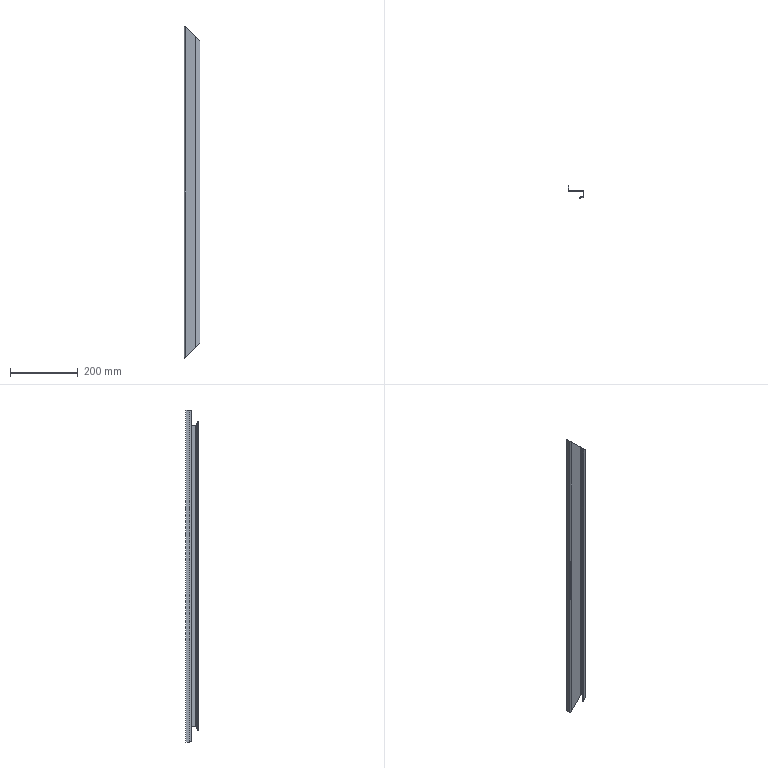Part | STEP file | 750038186 | 1 solid | 30 faces | box 47 x 35.779 x 981 mm | volume 158783 mm3 | plane 18 | cylinder 6 | spline 6 | commonest cylinder face diameters 4 x3 8 x3
STEP:
#1=CARTESIAN_POINT('',(43.,2.,-449.5));
#2=VERTEX_POINT('',#1);
#3=CARTESIAN_POINT('',(43.,2.,449.5));
#4=VERTEX_POINT('',#3);
#5=CARTESIAN_POINT('',(43.,2.,490.5));
#6=DIRECTION('',(0.,0.,1.));
#7=VECTOR('',#6,1000.);
#8=LINE('',#5,#7);
#9=EDGE_CURVE('',#2,#4,#8,.T.);
#10=ORIENTED_EDGE('',*,*,#9,.F.);
#11=CARTESIAN_POINT('',(4.,2.,-488.5));
#12=VERTEX_POINT('',#11);
#13=CARTESIAN_POINT('',(4.,2.,-488.5));
#14=DIRECTION('',(0.7071,0.,0.7071));
#15=VECTOR('',#14,1000.);
#16=LINE('',#13,#15);
#17=EDGE_CURVE('',#12,#2,#16,.T.);
#18=ORIENTED_EDGE('',*,*,#17,.F.);
#19=CARTESIAN_POINT('',(4.,2.,488.5));
#20=VERTEX_POINT('',#19);
#21=CARTESIAN_POINT('',(4.,2.,490.5));
#22=DIRECTION('',(0.,0.,-1.));
#23=VECTOR('',#22,1000.);
#24=LINE('',#21,#23);
#25=EDGE_CURVE('',#20,#12,#24,.T.);
#26=ORIENTED_EDGE('',*,*,#25,.F.);
#27=CARTESIAN_POINT('',(43.,2.,449.5));
#28=DIRECTION('',(-0.7071,0.,0.7071));
#29=VECTOR('',#28,1000.);
#30=LINE('',#27,#29);
#31=EDGE_CURVE('',#4,#20,#30,.T.);
#32=ORIENTED_EDGE('',*,*,#31,.F.);
#33=EDGE_LOOP('',(#10,#18,#26,#32));
#34=FACE_OUTER_BOUND('',#33,.T.);
#35=CARTESIAN_POINT('',(45.,2.,490.5));
#36=DIRECTION('',(0.,-1.,0.));
#37=DIRECTION('',(0.,0.,-1.));
#38=AXIS2_PLACEMENT_3D('',#35,#36,#37);
#39=PLANE('',#38);
#40=ADVANCED_FACE('',(#34),#39,.F.);
#41=CARTESIAN_POINT('',(43.,0.,449.5));
#42=VERTEX_POINT('',#41);
#43=CARTESIAN_POINT('',(43.,0.,449.5));
#44=DIRECTION('',(0.,1.,0.));
#45=VECTOR('',#44,1000.);
#46=LINE('',#43,#45);
#47=EDGE_CURVE('',#42,#4,#46,.T.);
#48=ORIENTED_EDGE('',*,*,#47,.T.);
#49=ORIENTED_EDGE('',*,*,#31,.T.);
#50=CARTESIAN_POINT('',(4.,0.,488.5));
#51=VERTEX_POINT('',#50);
#52=CARTESIAN_POINT('',(4.,0.,488.5));
#53=DIRECTION('',(0.,-1.,0.));
#54=VECTOR('',#53,1000.);
#55=LINE('',#52,#54);
#56=EDGE_CURVE('',#20,#51,#55,.T.);
#57=ORIENTED_EDGE('',*,*,#56,.T.);
#58=CARTESIAN_POINT('',(23.5,0.,469.));
#59=DIRECTION('',(0.7071,0.,-0.7071));
#60=VECTOR('',#59,1000.);
#61=LINE('',#58,#60);
#62=EDGE_CURVE('',#51,#42,#61,.T.);
#63=ORIENTED_EDGE('',*,*,#62,.T.);
#64=EDGE_LOOP('',(#48,#49,#57,#63));
#65=FACE_OUTER_BOUND('',#64,.T.);
#66=CARTESIAN_POINT('',(23.5,0.,469.));
#67=DIRECTION('',(0.7071,0.,0.7071));
#68=DIRECTION('',(0.7071,0.,-0.7071));
#69=AXIS2_PLACEMENT_3D('',#66,#67,#68);
#70=PLANE('',#69);
#71=ADVANCED_FACE('',(#65),#70,.T.);
#72=CARTESIAN_POINT('',(47.,-2.,-445.5));
#73=VERTEX_POINT('',#72);
#74=CARTESIAN_POINT('',(47.,-2.,-445.5));
#75=CARTESIAN_POINT('',(47.,0.,-445.5));
#76=CARTESIAN_POINT('',(45.667,2.,-446.833));
#77=CARTESIAN_POINT('',(43.,2.,-449.5));
#78=(BOUNDED_CURVE()B_SPLINE_CURVE(3,(#74,#75,#76,#77),.UNSPECIFIED.,.F.,.T.)B_SPLINE_CURVE_WITH_KNOTS((4,4),(0.,0.007635),.UNSPECIFIED.)CURVE()GEOMETRIC_REPRESENTATION_ITEM()RATIONAL_B_SPLINE_CURVE((1.,0.6667,0.5,0.5))REPRESENTATION_ITEM(''));
#79=EDGE_CURVE('',#73,#2,#78,.T.);
#80=ORIENTED_EDGE('',*,*,#79,.T.);
#81=ORIENTED_EDGE('',*,*,#9,.T.);
#82=CARTESIAN_POINT('',(47.,-2.,445.5));
#83=VERTEX_POINT('',#82);
#84=CARTESIAN_POINT('',(43.,2.,449.5));
#85=CARTESIAN_POINT('',(45.667,2.,446.833));
#86=CARTESIAN_POINT('',(47.,0.,445.5));
#87=CARTESIAN_POINT('',(47.,-2.,445.5));
#88=(BOUNDED_CURVE()B_SPLINE_CURVE(3,(#84,#85,#86,#87),.UNSPECIFIED.,.F.,.F.)B_SPLINE_CURVE_WITH_KNOTS((4,4),(0.,0.007567),.UNSPECIFIED.)CURVE()GEOMETRIC_REPRESENTATION_ITEM()RATIONAL_B_SPLINE_CURVE((0.5,0.5,0.6667,1.))REPRESENTATION_ITEM(''));
#89=EDGE_CURVE('',#4,#83,#88,.T.);
#90=ORIENTED_EDGE('',*,*,#89,.T.);
#91=CARTESIAN_POINT('',(47.,-2.,490.5));
#92=DIRECTION('',(0.,0.,-1.));
#93=VECTOR('',#92,1000.);
#94=LINE('',#91,#93);
#95=EDGE_CURVE('',#83,#73,#94,.T.);
#96=ORIENTED_EDGE('',*,*,#95,.T.);
#97=EDGE_LOOP('',(#80,#81,#90,#96));
#98=FACE_OUTER_BOUND('',#97,.T.);
#99=CARTESIAN_POINT('',(43.,-2.,490.5));
#100=DIRECTION('',(0.,0.,-1.));
#101=DIRECTION('',(-1.,0.,0.));
#102=AXIS2_PLACEMENT_3D('',#99,#100,#101);
#103=CYLINDRICAL_SURFACE('',#102,4.);
#104=ADVANCED_FACE('',(#98),#103,.T.);
#105=CARTESIAN_POINT('',(4.,0.,-488.5));
#106=VERTEX_POINT('',#105);
#107=CARTESIAN_POINT('',(4.,0.,-488.5));
#108=DIRECTION('',(0.,1.,0.));
#109=VECTOR('',#108,1000.);
#110=LINE('',#107,#109);
#111=EDGE_CURVE('',#106,#12,#110,.T.);
#112=ORIENTED_EDGE('',*,*,#111,.T.);
#113=ORIENTED_EDGE('',*,*,#17,.T.);
#114=CARTESIAN_POINT('',(43.,0.,-449.5));
#115=VERTEX_POINT('',#114);
#116=CARTESIAN_POINT('',(43.,0.,-449.5));
#117=DIRECTION('',(0.,-1.,0.));
#118=VECTOR('',#117,1000.);
#119=LINE('',#116,#118);
#120=EDGE_CURVE('',#2,#115,#119,.T.);
#121=ORIENTED_EDGE('',*,*,#120,.T.);
#122=CARTESIAN_POINT('',(514.,0.,21.5));
#123=DIRECTION('',(-0.7071,0.,-0.7071));
#124=VECTOR('',#123,1000.);
#125=LINE('',#122,#124);
#126=EDGE_CURVE('',#115,#106,#125,.T.);
#127=ORIENTED_EDGE('',*,*,#126,.T.);
#128=EDGE_LOOP('',(#112,#113,#121,#127));
#129=FACE_OUTER_BOUND('',#128,.T.);
#130=CARTESIAN_POINT('',(514.,0.,21.5));
#131=DIRECTION('',(0.7071,0.,-0.7071));
#132=DIRECTION('',(-0.7071,0.,-0.7071));
#133=AXIS2_PLACEMENT_3D('',#130,#131,#132);
#134=PLANE('',#133);
#135=ADVANCED_FACE('',(#129),#134,.T.);
#136=ORIENTED_EDGE('',*,*,#25,.T.);
#137=CARTESIAN_POINT('',(2.,4.,-490.5));
#138=VERTEX_POINT('',#137);
#139=CARTESIAN_POINT('',(2.,4.,-490.5));
#140=CARTESIAN_POINT('',(2.,3.,-490.5));
#141=CARTESIAN_POINT('',(2.667,2.,-489.833));
#142=CARTESIAN_POINT('',(4.,2.,-488.5));
#143=(BOUNDED_CURVE()B_SPLINE_CURVE(3,(#139,#140,#141,#142),.UNSPECIFIED.,.F.,.F.)B_SPLINE_CURVE_WITH_KNOTS((4,4),(0.,0.003806),.UNSPECIFIED.)CURVE()GEOMETRIC_REPRESENTATION_ITEM()RATIONAL_B_SPLINE_CURVE((1.,0.6667,0.5,0.5))REPRESENTATION_ITEM(''));
#144=EDGE_CURVE('',#138,#12,#143,.T.);
#145=ORIENTED_EDGE('',*,*,#144,.F.);
#146=CARTESIAN_POINT('',(2.,4.,490.5));
#147=VERTEX_POINT('',#146);
#148=CARTESIAN_POINT('',(2.,4.,490.5));
#149=DIRECTION('',(0.,0.,-1.));
#150=VECTOR('',#149,1000.);
#151=LINE('',#148,#150);
#152=EDGE_CURVE('',#147,#138,#151,.T.);
#153=ORIENTED_EDGE('',*,*,#152,.F.);
#154=CARTESIAN_POINT('',(4.,2.,488.5));
#155=CARTESIAN_POINT('',(2.667,2.,489.833));
#156=CARTESIAN_POINT('',(2.,3.,490.5));
#157=CARTESIAN_POINT('',(2.,4.,490.5));
#158=(BOUNDED_CURVE()B_SPLINE_CURVE(3,(#154,#155,#156,#157),.UNSPECIFIED.,.F.,.F.)B_SPLINE_CURVE_WITH_KNOTS((4,4),(0.,0.003785),.UNSPECIFIED.)CURVE()GEOMETRIC_REPRESENTATION_ITEM()RATIONAL_B_SPLINE_CURVE((0.5,0.5,0.6667,1.))REPRESENTATION_ITEM(''));
#159=EDGE_CURVE('',#20,#147,#158,.T.);
#160=ORIENTED_EDGE('',*,*,#159,.F.);
#161=EDGE_LOOP('',(#136,#145,#153,#160));
#162=FACE_OUTER_BOUND('',#161,.T.);
#163=CARTESIAN_POINT('',(4.,4.,490.5));
#164=DIRECTION('',(0.,0.,-1.));
#165=DIRECTION('',(-1.,0.,0.));
#166=AXIS2_PLACEMENT_3D('',#163,#164,#165);
#167=CYLINDRICAL_SURFACE('',#166,2.);
#168=ADVANCED_FACE('',(#162),#167,.F.);
#169=ORIENTED_EDGE('',*,*,#89,.F.);
#170=ORIENTED_EDGE('',*,*,#47,.F.);
#171=CARTESIAN_POINT('',(45.,-2.,445.5));
#172=VERTEX_POINT('',#171);
#173=CARTESIAN_POINT('',(45.,-2.,445.5));
#174=CARTESIAN_POINT('',(45.,-1.,445.5));
#175=CARTESIAN_POINT('',(44.333,0.,446.833));
#176=CARTESIAN_POINT('',(43.,0.,449.5));
#177=(BOUNDED_CURVE()B_SPLINE_CURVE(3,(#173,#174,#175,#176),.UNSPECIFIED.,.F.,.T.)B_SPLINE_CURVE_WITH_KNOTS((4,4),(0.,0.00529),.UNSPECIFIED.)CURVE()GEOMETRIC_REPRESENTATION_ITEM()RATIONAL_B_SPLINE_CURVE((1.,0.6667,0.5,0.5))REPRESENTATION_ITEM(''));
#178=EDGE_CURVE('',#172,#42,#177,.T.);
#179=ORIENTED_EDGE('',*,*,#178,.F.);
#180=CARTESIAN_POINT('',(46.,-2.,445.5));
#181=DIRECTION('',(-1.,0.,0.));
#182=VECTOR('',#181,1000.);
#183=LINE('',#180,#182);
#184=EDGE_CURVE('',#83,#172,#183,.T.);
#185=ORIENTED_EDGE('',*,*,#184,.F.);
#186=EDGE_LOOP('',(#169,#170,#179,#185));
#187=FACE_OUTER_BOUND('',#186,.T.);
#188=CARTESIAN_POINT('',(45.,-2.,445.5));
#189=CARTESIAN_POINT('',(45.667,-2.,445.5));
#190=CARTESIAN_POINT('',(46.333,-2.,445.5));
#191=CARTESIAN_POINT('',(47.,-2.,445.5));
#192=CARTESIAN_POINT('',(45.,2.,445.5));
#193=CARTESIAN_POINT('',(45.667,3.333,445.5));
#194=CARTESIAN_POINT('',(46.333,4.667,445.5));
#195=CARTESIAN_POINT('',(47.,6.,445.5));
#196=CARTESIAN_POINT('',(41.,2.,453.5));
#197=CARTESIAN_POINT('',(40.333,3.333,453.5));
#198=CARTESIAN_POINT('',(39.667,4.667,453.5));
#199=CARTESIAN_POINT('',(39.,6.,453.5));
#200=CARTESIAN_POINT('',(41.,-2.,453.5));
#201=CARTESIAN_POINT('',(40.333,-2.,453.5));
#202=CARTESIAN_POINT('',(39.667,-2.,453.5));
#203=CARTESIAN_POINT('',(39.,-2.,453.5));
#204=CARTESIAN_POINT('',(41.,-6.,453.5));
#205=CARTESIAN_POINT('',(40.333,-7.333,453.5));
#206=CARTESIAN_POINT('',(39.667,-8.667,453.5));
#207=CARTESIAN_POINT('',(39.,-10.,453.5));
#208=CARTESIAN_POINT('',(45.,-6.,445.5));
#209=CARTESIAN_POINT('',(45.667,-7.333,445.5));
#210=CARTESIAN_POINT('',(46.333,-8.667,445.5));
#211=CARTESIAN_POINT('',(47.,-10.,445.5));
#212=CARTESIAN_POINT('',(45.,-2.,445.5));
#213=CARTESIAN_POINT('',(45.667,-2.,445.5));
#214=CARTESIAN_POINT('',(46.333,-2.,445.5));
#215=CARTESIAN_POINT('',(47.,-2.,445.5));
#216=(BOUNDED_SURFACE()B_SPLINE_SURFACE(3,3,((#188,#189,#190,#191),(#192,#193,#194,#195),(#196,#197,#198,#199),(#200,#201,#202,#203),(#204,#205,#206,#207),(#208,#209,#210,#211),(#212,#213,#214,#215)),.UNSPECIFIED.,.T.,.F.,.F.)B_SPLINE_SURFACE_WITH_KNOTS((4,3,4),(4,4),(0.,0.5,1.),(0.,1.),.UNSPECIFIED.)GEOMETRIC_REPRESENTATION_ITEM()RATIONAL_B_SPLINE_SURFACE(((1.,1.,1.,1.),(0.3333,0.3333,0.3333,0.3333),(0.3333,0.3333,0.3333,0.3333),(1.,1.,1.,1.),(0.3333,0.3333,0.3333,0.3333),(0.3333,0.3333,0.3333,0.3333),(1.,1.,1.,1.)))REPRESENTATION_ITEM('')SURFACE());
#217=ADVANCED_FACE('',(#187),#216,.F.);
#218=CARTESIAN_POINT('',(4.,0.,490.5));
#219=DIRECTION('',(0.,0.,-1.));
#220=VECTOR('',#219,1000.);
#221=LINE('',#218,#220);
#222=EDGE_CURVE('',#51,#106,#221,.T.);
#223=ORIENTED_EDGE('',*,*,#222,.T.);
#224=ORIENTED_EDGE('',*,*,#126,.F.);
#225=CARTESIAN_POINT('',(43.,0.,490.5));
#226=DIRECTION('',(0.,0.,1.));
#227=VECTOR('',#226,1000.);
#228=LINE('',#225,#227);
#229=EDGE_CURVE('',#115,#42,#228,.T.);
#230=ORIENTED_EDGE('',*,*,#229,.T.);
#231=ORIENTED_EDGE('',*,*,#62,.F.);
#232=EDGE_LOOP('',(#223,#224,#230,#231));
#233=FACE_OUTER_BOUND('',#232,.T.);
#234=CARTESIAN_POINT('',(45.,0.,490.5));
#235=DIRECTION('',(0.,-1.,0.));
#236=DIRECTION('',(0.,0.,-1.));
#237=AXIS2_PLACEMENT_3D('',#234,#235,#236);
#238=PLANE('',#237);
#239=ADVANCED_FACE('',(#233),#238,.T.);
#240=ORIENTED_EDGE('',*,*,#56,.F.);
#241=ORIENTED_EDGE('',*,*,#159,.T.);
#242=CARTESIAN_POINT('',(0.,4.,490.5));
#243=VERTEX_POINT('',#242);
#244=CARTESIAN_POINT('',(1.,4.,490.5));
#245=DIRECTION('',(1.,0.,0.));
#246=VECTOR('',#245,1000.);
#247=LINE('',#244,#246);
#248=EDGE_CURVE('',#243,#147,#247,.T.);
#249=ORIENTED_EDGE('',*,*,#248,.F.);
#250=CARTESIAN_POINT('',(4.,0.,488.5));
#251=CARTESIAN_POINT('',(1.333,0.,489.833));
#252=CARTESIAN_POINT('',(0.,2.,490.5));
#253=CARTESIAN_POINT('',(0.,4.,490.5));
#254=(BOUNDED_CURVE()B_SPLINE_CURVE(3,(#250,#251,#252,#253),.UNSPECIFIED.,.F.,.T.)B_SPLINE_CURVE_WITH_KNOTS((4,4),(0.,0.006641),.UNSPECIFIED.)CURVE()GEOMETRIC_REPRESENTATION_ITEM()RATIONAL_B_SPLINE_CURVE((0.5,0.5,0.6667,1.))REPRESENTATION_ITEM(''));
#255=EDGE_CURVE('',#51,#243,#254,.T.);
#256=ORIENTED_EDGE('',*,*,#255,.F.);
#257=EDGE_LOOP('',(#240,#241,#249,#256));
#258=FACE_OUTER_BOUND('',#257,.T.);
#259=CARTESIAN_POINT('',(8.,4.,486.5));
#260=CARTESIAN_POINT('',(7.333,4.,486.5));
#261=CARTESIAN_POINT('',(6.667,4.,486.5));
#262=CARTESIAN_POINT('',(6.,4.,486.5));
#263=CARTESIAN_POINT('',(8.,-4.,486.5));
#264=CARTESIAN_POINT('',(7.333,-2.667,486.5));
#265=CARTESIAN_POINT('',(6.667,-1.333,486.5));
#266=CARTESIAN_POINT('',(6.,0.,486.5));
#267=CARTESIAN_POINT('',(0.,-4.,490.5));
#268=CARTESIAN_POINT('',(0.6667,-2.667,490.5));
#269=CARTESIAN_POINT('',(1.333,-1.333,490.5));
#270=CARTESIAN_POINT('',(2.,0.,490.5));
#271=CARTESIAN_POINT('',(0.,4.,490.5));
#272=CARTESIAN_POINT('',(0.6667,4.,490.5));
#273=CARTESIAN_POINT('',(1.333,4.,490.5));
#274=CARTESIAN_POINT('',(2.,4.,490.5));
#275=CARTESIAN_POINT('',(0.,12.,490.5));
#276=CARTESIAN_POINT('',(0.6667,10.667,490.5));
#277=CARTESIAN_POINT('',(1.333,9.333,490.5));
#278=CARTESIAN_POINT('',(2.,8.,490.5));
#279=CARTESIAN_POINT('',(8.,12.,486.5));
#280=CARTESIAN_POINT('',(7.333,10.667,486.5));
#281=CARTESIAN_POINT('',(6.667,9.333,486.5));
#282=CARTESIAN_POINT('',(6.,8.,486.5));
#283=CARTESIAN_POINT('',(8.,4.,486.5));
#284=CARTESIAN_POINT('',(7.333,4.,486.5));
#285=CARTESIAN_POINT('',(6.667,4.,486.5));
#286=CARTESIAN_POINT('',(6.,4.,486.5));
#287=(BOUNDED_SURFACE()B_SPLINE_SURFACE(3,3,((#259,#260,#261,#262),(#263,#264,#265,#266),(#267,#268,#269,#270),(#271,#272,#273,#274),(#275,#276,#277,#278),(#279,#280,#281,#282),(#283,#284,#285,#286)),.UNSPECIFIED.,.T.,.F.,.F.)B_SPLINE_SURFACE_WITH_KNOTS((4,3,4),(4,4),(0.,0.5,1.),(0.,1.),.UNSPECIFIED.)GEOMETRIC_REPRESENTATION_ITEM()RATIONAL_B_SPLINE_SURFACE(((1.,1.,1.,1.),(0.3333,0.3333,0.3333,0.3333),(0.3333,0.3333,0.3333,0.3333),(1.,1.,1.,1.),(0.3333,0.3333,0.3333,0.3333),(0.3333,0.3333,0.3333,0.3333),(1.,1.,1.,1.)))REPRESENTATION_ITEM('')SURFACE());
#288=ADVANCED_FACE('',(#258),#287,.F.);
#289=ORIENTED_EDGE('',*,*,#79,.F.);
#290=CARTESIAN_POINT('',(45.,-2.,-445.5));
#291=VERTEX_POINT('',#290);
#292=CARTESIAN_POINT('',(46.,-2.,-445.5));
#293=DIRECTION('',(1.,0.,0.));
#294=VECTOR('',#293,1000.);
#295=LINE('',#292,#294);
#296=EDGE_CURVE('',#291,#73,#295,.T.);
#297=ORIENTED_EDGE('',*,*,#296,.F.);
#298=CARTESIAN_POINT('',(43.,0.,-449.5));
#299=CARTESIAN_POINT('',(44.333,0.,-446.833));
#300=CARTESIAN_POINT('',(45.,-1.,-445.5));
#301=CARTESIAN_POINT('',(45.,-2.,-445.5));
#302=(BOUNDED_CURVE()B_SPLINE_CURVE(3,(#298,#299,#300,#301),.UNSPECIFIED.,.F.,.T.)B_SPLINE_CURVE_WITH_KNOTS((4,4),(0.,0.005228),.UNSPECIFIED.)CURVE()GEOMETRIC_REPRESENTATION_ITEM()RATIONAL_B_SPLINE_CURVE((0.5,0.5,0.6667,1.))REPRESENTATION_ITEM(''));
#303=EDGE_CURVE('',#115,#291,#302,.T.);
#304=ORIENTED_EDGE('',*,*,#303,.F.);
#305=ORIENTED_EDGE('',*,*,#120,.F.);
#306=EDGE_LOOP('',(#289,#297,#304,#305));
#307=FACE_OUTER_BOUND('',#306,.T.);
#308=CARTESIAN_POINT('',(41.,-2.,-453.5));
#309=CARTESIAN_POINT('',(40.333,-2.,-453.5));
#310=CARTESIAN_POINT('',(39.667,-2.,-453.5));
#311=CARTESIAN_POINT('',(39.,-2.,-453.5));
#312=CARTESIAN_POINT('',(41.,2.,-453.5));
#313=CARTESIAN_POINT('',(40.333,3.333,-453.5));
#314=CARTESIAN_POINT('',(39.667,4.667,-453.5));
#315=CARTESIAN_POINT('',(39.,6.,-453.5));
#316=CARTESIAN_POINT('',(45.,2.,-445.5));
#317=CARTESIAN_POINT('',(45.667,3.333,-445.5));
#318=CARTESIAN_POINT('',(46.333,4.667,-445.5));
#319=CARTESIAN_POINT('',(47.,6.,-445.5));
#320=CARTESIAN_POINT('',(45.,-2.,-445.5));
#321=CARTESIAN_POINT('',(45.667,-2.,-445.5));
#322=CARTESIAN_POINT('',(46.333,-2.,-445.5));
#323=CARTESIAN_POINT('',(47.,-2.,-445.5));
#324=CARTESIAN_POINT('',(45.,-6.,-445.5));
#325=CARTESIAN_POINT('',(45.667,-7.333,-445.5));
#326=CARTESIAN_POINT('',(46.333,-8.667,-445.5));
#327=CARTESIAN_POINT('',(47.,-10.,-445.5));
#328=CARTESIAN_POINT('',(41.,-6.,-453.5));
#329=CARTESIAN_POINT('',(40.333,-7.333,-453.5));
#330=CARTESIAN_POINT('',(39.667,-8.667,-453.5));
#331=CARTESIAN_POINT('',(39.,-10.,-453.5));
#332=CARTESIAN_POINT('',(41.,-2.,-453.5));
#333=CARTESIAN_POINT('',(40.333,-2.,-453.5));
#334=CARTESIAN_POINT('',(39.667,-2.,-453.5));
#335=CARTESIAN_POINT('',(39.,-2.,-453.5));
#336=(BOUNDED_SURFACE()B_SPLINE_SURFACE(3,3,((#308,#309,#310,#311),(#312,#313,#314,#315),(#316,#317,#318,#319),(#320,#321,#322,#323),(#324,#325,#326,#327),(#328,#329,#330,#331),(#332,#333,#334,#335)),.UNSPECIFIED.,.T.,.F.,.F.)B_SPLINE_SURFACE_WITH_KNOTS((4,3,4),(4,4),(0.,0.5,1.),(0.,1.),.UNSPECIFIED.)GEOMETRIC_REPRESENTATION_ITEM()RATIONAL_B_SPLINE_SURFACE(((1.,1.,1.,1.),(0.3333,0.3333,0.3333,0.3333),(0.3333,0.3333,0.3333,0.3333),(1.,1.,1.,1.),(0.3333,0.3333,0.3333,0.3333),(0.3333,0.3333,0.3333,0.3333),(1.,1.,1.,1.)))REPRESENTATION_ITEM('')SURFACE());
#337=ADVANCED_FACE('',(#307),#336,.F.);
#338=CARTESIAN_POINT('',(47.,-14.465,-445.5));
#339=VERTEX_POINT('',#338);
#340=CARTESIAN_POINT('',(47.,-14.465,445.5));
#341=VERTEX_POINT('',#340);
#342=CARTESIAN_POINT('',(47.,-14.465,490.5));
#343=DIRECTION('',(0.,0.,1.));
#344=VECTOR('',#343,1000.);
#345=LINE('',#342,#344);
#346=EDGE_CURVE('',#339,#341,#345,.T.);
#347=ORIENTED_EDGE('',*,*,#346,.F.);
#348=CARTESIAN_POINT('',(47.,-16.,-445.5));
#349=DIRECTION('',(0.,-1.,0.));
#350=VECTOR('',#349,1000.);
#351=LINE('',#348,#350);
#352=EDGE_CURVE('',#73,#339,#351,.T.);
#353=ORIENTED_EDGE('',*,*,#352,.F.);
#354=ORIENTED_EDGE('',*,*,#95,.F.);
#355=CARTESIAN_POINT('',(47.,-16.,445.5));
#356=DIRECTION('',(0.,1.,0.));
#357=VECTOR('',#356,1000.);
#358=LINE('',#355,#357);
#359=EDGE_CURVE('',#341,#83,#358,.T.);
#360=ORIENTED_EDGE('',*,*,#359,.F.);
#361=EDGE_LOOP('',(#347,#353,#354,#360));
#362=FACE_OUTER_BOUND('',#361,.T.);
#363=CARTESIAN_POINT('',(47.,-16.,490.5));
#364=DIRECTION('',(-1.,0.,0.));
#365=DIRECTION('',(0.,-1.,0.));
#366=AXIS2_PLACEMENT_3D('',#363,#364,#365);
#367=PLANE('',#366);
#368=ADVANCED_FACE('',(#362),#367,.F.);
#369=ORIENTED_EDGE('',*,*,#144,.T.);
#370=ORIENTED_EDGE('',*,*,#111,.F.);
#371=CARTESIAN_POINT('',(0.,4.,-490.5));
#372=VERTEX_POINT('',#371);
#373=CARTESIAN_POINT('',(0.,4.,-490.5));
#374=CARTESIAN_POINT('',(0.,2.,-490.5));
#375=CARTESIAN_POINT('',(1.333,0.,-489.833));
#376=CARTESIAN_POINT('',(4.,0.,-488.5));
#377=(BOUNDED_CURVE()B_SPLINE_CURVE(3,(#373,#374,#375,#376),.UNSPECIFIED.,.F.,.F.)B_SPLINE_CURVE_WITH_KNOTS((4,4),(0.,0.006627),.UNSPECIFIED.)CURVE()GEOMETRIC_REPRESENTATION_ITEM()RATIONAL_B_SPLINE_CURVE((1.,0.6667,0.5,0.5))REPRESENTATION_ITEM(''));
#378=EDGE_CURVE('',#372,#106,#377,.T.);
#379=ORIENTED_EDGE('',*,*,#378,.F.);
#380=CARTESIAN_POINT('',(1.,4.,-490.5));
#381=DIRECTION('',(-1.,0.,0.));
#382=VECTOR('',#381,1000.);
#383=LINE('',#380,#382);
#384=EDGE_CURVE('',#138,#372,#383,.T.);
#385=ORIENTED_EDGE('',*,*,#384,.F.);
#386=EDGE_LOOP('',(#369,#370,#379,#385));
#387=FACE_OUTER_BOUND('',#386,.T.);
#388=CARTESIAN_POINT('',(0.,4.,-490.5));
#389=CARTESIAN_POINT('',(0.6667,4.,-490.5));
#390=CARTESIAN_POINT('',(1.333,4.,-490.5));
#391=CARTESIAN_POINT('',(2.,4.,-490.5));
#392=CARTESIAN_POINT('',(0.,-4.,-490.5));
#393=CARTESIAN_POINT('',(0.6667,-2.667,-490.5));
#394=CARTESIAN_POINT('',(1.333,-1.333,-490.5));
#395=CARTESIAN_POINT('',(2.,0.,-490.5));
#396=CARTESIAN_POINT('',(8.,-4.,-486.5));
#397=CARTESIAN_POINT('',(7.333,-2.667,-486.5));
#398=CARTESIAN_POINT('',(6.667,-1.333,-486.5));
#399=CARTESIAN_POINT('',(6.,0.,-486.5));
#400=CARTESIAN_POINT('',(8.,4.,-486.5));
#401=CARTESIAN_POINT('',(7.333,4.,-486.5));
#402=CARTESIAN_POINT('',(6.667,4.,-486.5));
#403=CARTESIAN_POINT('',(6.,4.,-486.5));
#404=CARTESIAN_POINT('',(8.,12.,-486.5));
#405=CARTESIAN_POINT('',(7.333,10.667,-486.5));
#406=CARTESIAN_POINT('',(6.667,9.333,-486.5));
#407=CARTESIAN_POINT('',(6.,8.,-486.5));
#408=CARTESIAN_POINT('',(0.,12.,-490.5));
#409=CARTESIAN_POINT('',(0.6667,10.667,-490.5));
#410=CARTESIAN_POINT('',(1.333,9.333,-490.5));
#411=CARTESIAN_POINT('',(2.,8.,-490.5));
#412=CARTESIAN_POINT('',(0.,4.,-490.5));
#413=CARTESIAN_POINT('',(0.6667,4.,-490.5));
#414=CARTESIAN_POINT('',(1.333,4.,-490.5));
#415=CARTESIAN_POINT('',(2.,4.,-490.5));
#416=(BOUNDED_SURFACE()B_SPLINE_SURFACE(3,3,((#388,#389,#390,#391),(#392,#393,#394,#395),(#396,#397,#398,#399),(#400,#401,#402,#403),(#404,#405,#406,#407),(#408,#409,#410,#411),(#412,#413,#414,#415)),.UNSPECIFIED.,.T.,.F.,.T.)B_SPLINE_SURFACE_WITH_KNOTS((4,3,4),(4,4),(0.,0.5,1.),(0.,1.),.UNSPECIFIED.)GEOMETRIC_REPRESENTATION_ITEM()RATIONAL_B_SPLINE_SURFACE(((1.,1.,1.,1.),(0.3333,0.3333,0.3333,0.3333),(0.3333,0.3333,0.3333,0.3333),(1.,1.,1.,1.),(0.3333,0.3333,0.3333,0.3333),(0.3333,0.3333,0.3333,0.3333),(1.,1.,1.,1.)))REPRESENTATION_ITEM('')SURFACE());
#417=ADVANCED_FACE('',(#387),#416,.F.);
#418=CARTESIAN_POINT('',(2.,15.,490.5));
#419=VERTEX_POINT('',#418);
#420=CARTESIAN_POINT('',(2.,15.,-490.5));
#421=VERTEX_POINT('',#420);
#422=CARTESIAN_POINT('',(2.,15.,490.5));
#423=DIRECTION('',(0.,0.,-1.));
#424=VECTOR('',#423,1000.);
#425=LINE('',#422,#424);
#426=EDGE_CURVE('',#419,#421,#425,.T.);
#427=ORIENTED_EDGE('',*,*,#426,.F.);
#428=CARTESIAN_POINT('',(2.,0.,490.5));
#429=DIRECTION('',(0.,1.,0.));
#430=VECTOR('',#429,1000.);
#431=LINE('',#428,#430);
#432=EDGE_CURVE('',#147,#419,#431,.T.);
#433=ORIENTED_EDGE('',*,*,#432,.F.);
#434=ORIENTED_EDGE('',*,*,#152,.T.);
#435=CARTESIAN_POINT('',(2.,0.,-490.5));
#436=DIRECTION('',(0.,-1.,0.));
#437=VECTOR('',#436,1000.);
#438=LINE('',#435,#437);
#439=EDGE_CURVE('',#421,#138,#438,.T.);
#440=ORIENTED_EDGE('',*,*,#439,.F.);
#441=EDGE_LOOP('',(#427,#433,#434,#440));
#442=FACE_OUTER_BOUND('',#441,.T.);
#443=CARTESIAN_POINT('',(2.,0.,490.5));
#444=DIRECTION('',(-1.,0.,0.));
#445=DIRECTION('',(0.,-1.,0.));
#446=AXIS2_PLACEMENT_3D('',#443,#444,#445);
#447=PLANE('',#446);
#448=ADVANCED_FACE('',(#442),#447,.F.);
#449=ORIENTED_EDGE('',*,*,#184,.T.);
#450=CARTESIAN_POINT('',(45.,-14.465,445.5));
#451=VERTEX_POINT('',#450);
#452=CARTESIAN_POINT('',(45.,-16.,445.5));
#453=DIRECTION('',(0.,-1.,0.));
#454=VECTOR('',#453,1000.);
#455=LINE('',#452,#454);
#456=EDGE_CURVE('',#172,#451,#455,.T.);
#457=ORIENTED_EDGE('',*,*,#456,.T.);
#458=CARTESIAN_POINT('',(47.,-14.465,445.5));
#459=DIRECTION('',(1.,0.,0.));
#460=VECTOR('',#459,1000.);
#461=LINE('',#458,#460);
#462=EDGE_CURVE('',#451,#341,#461,.T.);
#463=ORIENTED_EDGE('',*,*,#462,.T.);
#464=ORIENTED_EDGE('',*,*,#359,.T.);
#465=EDGE_LOOP('',(#449,#457,#463,#464));
#466=FACE_OUTER_BOUND('',#465,.T.);
#467=CARTESIAN_POINT('',(47.,-16.,445.5));
#468=DIRECTION('',(0.,0.,1.));
#469=DIRECTION('',(0.,-1.,0.));
#470=AXIS2_PLACEMENT_3D('',#467,#468,#469);
#471=PLANE('',#470);
#472=ADVANCED_FACE('',(#466),#471,.T.);
#473=ORIENTED_EDGE('',*,*,#178,.T.);
#474=ORIENTED_EDGE('',*,*,#229,.F.);
#475=ORIENTED_EDGE('',*,*,#303,.T.);
#476=CARTESIAN_POINT('',(45.,-2.,490.5));
#477=DIRECTION('',(0.,0.,-1.));
#478=VECTOR('',#477,1000.);
#479=LINE('',#476,#478);
#480=EDGE_CURVE('',#172,#291,#479,.T.);
#481=ORIENTED_EDGE('',*,*,#480,.F.);
#482=EDGE_LOOP('',(#473,#474,#475,#481));
#483=FACE_OUTER_BOUND('',#482,.T.);
#484=CARTESIAN_POINT('',(43.,-2.,490.5));
#485=DIRECTION('',(0.,0.,-1.));
#486=DIRECTION('',(-1.,0.,0.));
#487=AXIS2_PLACEMENT_3D('',#484,#485,#486);
#488=CYLINDRICAL_SURFACE('',#487,2.);
#489=ADVANCED_FACE('',(#483),#488,.F.);
#490=CARTESIAN_POINT('',(0.,4.,490.5));
#491=DIRECTION('',(0.,0.,-1.));
#492=VECTOR('',#491,1000.);
#493=LINE('',#490,#492);
#494=EDGE_CURVE('',#243,#372,#493,.T.);
#495=ORIENTED_EDGE('',*,*,#494,.T.);
#496=ORIENTED_EDGE('',*,*,#378,.T.);
#497=ORIENTED_EDGE('',*,*,#222,.F.);
#498=ORIENTED_EDGE('',*,*,#255,.T.);
#499=EDGE_LOOP('',(#495,#496,#497,#498));
#500=FACE_OUTER_BOUND('',#499,.T.);
#501=CARTESIAN_POINT('',(4.,4.,490.5));
#502=DIRECTION('',(0.,0.,-1.));
#503=DIRECTION('',(-1.,0.,0.));
#504=AXIS2_PLACEMENT_3D('',#501,#502,#503);
#505=CYLINDRICAL_SURFACE('',#504,4.);
#506=ADVANCED_FACE('',(#500),#505,.T.);
#507=ORIENTED_EDGE('',*,*,#432,.T.);
#508=CARTESIAN_POINT('',(0.,15.,490.5));
#509=VERTEX_POINT('',#508);
#510=CARTESIAN_POINT('',(0.,15.,490.5));
#511=DIRECTION('',(-1.,0.,0.));
#512=VECTOR('',#511,1000.);
#513=LINE('',#510,#512);
#514=EDGE_CURVE('',#419,#509,#513,.T.);
#515=ORIENTED_EDGE('',*,*,#514,.T.);
#516=CARTESIAN_POINT('',(0.,0.,490.5));
#517=DIRECTION('',(0.,-1.,0.));
#518=VECTOR('',#517,1000.);
#519=LINE('',#516,#518);
#520=EDGE_CURVE('',#509,#243,#519,.T.);
#521=ORIENTED_EDGE('',*,*,#520,.T.);
#522=ORIENTED_EDGE('',*,*,#248,.T.);
#523=EDGE_LOOP('',(#507,#515,#521,#522));
#524=FACE_OUTER_BOUND('',#523,.T.);
#525=CARTESIAN_POINT('',(0.,0.,490.5));
#526=DIRECTION('',(0.,0.,1.));
#527=DIRECTION('',(1.,0.,0.));
#528=AXIS2_PLACEMENT_3D('',#525,#526,#527);
#529=PLANE('',#528);
#530=ADVANCED_FACE('',(#524),#529,.T.);
#531=CARTESIAN_POINT('',(45.,-14.465,-445.5));
#532=VERTEX_POINT('',#531);
#533=CARTESIAN_POINT('',(47.,-14.465,-445.5));
#534=DIRECTION('',(-1.,0.,0.));
#535=VECTOR('',#534,1000.);
#536=LINE('',#533,#535);
#537=EDGE_CURVE('',#339,#532,#536,.T.);
#538=ORIENTED_EDGE('',*,*,#537,.T.);
#539=CARTESIAN_POINT('',(45.,-16.,-445.5));
#540=DIRECTION('',(0.,1.,0.));
#541=VECTOR('',#540,1000.);
#542=LINE('',#539,#541);
#543=EDGE_CURVE('',#532,#291,#542,.T.);
#544=ORIENTED_EDGE('',*,*,#543,.T.);
#545=ORIENTED_EDGE('',*,*,#296,.T.);
#546=ORIENTED_EDGE('',*,*,#352,.T.);
#547=EDGE_LOOP('',(#538,#544,#545,#546));
#548=FACE_OUTER_BOUND('',#547,.T.);
#549=CARTESIAN_POINT('',(47.,-16.,-445.5));
#550=DIRECTION('',(0.,0.,-1.));
#551=DIRECTION('',(0.,1.,0.));
#552=AXIS2_PLACEMENT_3D('',#549,#550,#551);
#553=PLANE('',#552);
#554=ADVANCED_FACE('',(#548),#553,.T.);
#555=CARTESIAN_POINT('',(44.035,-18.329,-448.465));
#556=VERTEX_POINT('',#555);
#557=CARTESIAN_POINT('',(44.035,-18.329,-448.465));
#558=CARTESIAN_POINT('',(46.081,-17.781,-446.419));
#559=CARTESIAN_POINT('',(47.,-16.095,-445.5));
#560=CARTESIAN_POINT('',(47.,-14.465,-445.5));
#561=(BOUNDED_CURVE()B_SPLINE_CURVE(3,(#557,#558,#559,#560),.UNSPECIFIED.,.F.,.F.)B_SPLINE_CURVE_WITH_KNOTS((4,4),(0.,0.006101),.UNSPECIFIED.)CURVE()GEOMETRIC_REPRESENTATION_ITEM()RATIONAL_B_SPLINE_CURVE((0.5087,0.5468,0.7106,1.))REPRESENTATION_ITEM(''));
#562=EDGE_CURVE('',#556,#339,#561,.T.);
#563=ORIENTED_EDGE('',*,*,#562,.T.);
#564=ORIENTED_EDGE('',*,*,#346,.T.);
#565=CARTESIAN_POINT('',(44.035,-18.329,448.465));
#566=VERTEX_POINT('',#565);
#567=CARTESIAN_POINT('',(47.,-14.465,445.5));
#568=CARTESIAN_POINT('',(47.,-16.095,445.5));
#569=CARTESIAN_POINT('',(46.081,-17.781,446.419));
#570=CARTESIAN_POINT('',(44.035,-18.329,448.465));
#571=(BOUNDED_CURVE()B_SPLINE_CURVE(3,(#567,#568,#569,#570),.UNSPECIFIED.,.F.,.F.)B_SPLINE_CURVE_WITH_KNOTS((4,4),(0.,0.006218),.UNSPECIFIED.)CURVE()GEOMETRIC_REPRESENTATION_ITEM()RATIONAL_B_SPLINE_CURVE((1.,0.7106,0.5468,0.5087))REPRESENTATION_ITEM(''));
#572=EDGE_CURVE('',#341,#566,#571,.T.);
#573=ORIENTED_EDGE('',*,*,#572,.T.);
#574=CARTESIAN_POINT('',(44.035,-18.329,490.5));
#575=DIRECTION('',(0.,0.,-1.));
#576=VECTOR('',#575,1000.);
#577=LINE('',#574,#576);
#578=EDGE_CURVE('',#566,#556,#577,.T.);
#579=ORIENTED_EDGE('',*,*,#578,.T.);
#580=EDGE_LOOP('',(#563,#564,#573,#579));
#581=FACE_OUTER_BOUND('',#580,.T.);
#582=CARTESIAN_POINT('',(43.,-14.465,490.5));
#583=DIRECTION('',(0.,0.,-1.));
#584=DIRECTION('',(-1.,0.,0.));
#585=AXIS2_PLACEMENT_3D('',#582,#583,#584);
#586=CYLINDRICAL_SURFACE('',#585,4.);
#587=ADVANCED_FACE('',(#581),#586,.T.);
#588=CARTESIAN_POINT('',(0.,15.,-490.5));
#589=VERTEX_POINT('',#588);
#590=CARTESIAN_POINT('',(0.,-18.847,-490.5));
#591=DIRECTION('',(0.,-1.,0.));
#592=VECTOR('',#591,1000.);
#593=LINE('',#590,#592);
#594=EDGE_CURVE('',#589,#372,#593,.T.);
#595=ORIENTED_EDGE('',*,*,#594,.F.);
#596=CARTESIAN_POINT('',(34.375,15.,-490.5));
#597=DIRECTION('',(-1.,0.,0.));
#598=VECTOR('',#597,1000.);
#599=LINE('',#596,#598);
#600=EDGE_CURVE('',#421,#589,#599,.T.);
#601=ORIENTED_EDGE('',*,*,#600,.F.);
#602=ORIENTED_EDGE('',*,*,#439,.T.);
#603=ORIENTED_EDGE('',*,*,#384,.T.);
#604=EDGE_LOOP('',(#595,#601,#602,#603));
#605=FACE_OUTER_BOUND('',#604,.T.);
#606=CARTESIAN_POINT('',(34.375,-18.847,-490.5));
#607=DIRECTION('',(0.,0.,1.));
#608=DIRECTION('',(1.,0.,0.));
#609=AXIS2_PLACEMENT_3D('',#606,#607,#608);
#610=PLANE('',#609);
#611=ADVANCED_FACE('',(#605),#610,.F.);
#612=ORIENTED_EDGE('',*,*,#600,.T.);
#613=CARTESIAN_POINT('',(0.,15.,490.5));
#614=DIRECTION('',(0.,0.,1.));
#615=VECTOR('',#614,1000.);
#616=LINE('',#613,#615);
#617=EDGE_CURVE('',#589,#509,#616,.T.);
#618=ORIENTED_EDGE('',*,*,#617,.T.);
#619=ORIENTED_EDGE('',*,*,#514,.F.);
#620=ORIENTED_EDGE('',*,*,#426,.T.);
#621=EDGE_LOOP('',(#612,#618,#619,#620));
#622=FACE_OUTER_BOUND('',#621,.T.);
#623=CARTESIAN_POINT('',(0.,15.,490.5));
#624=DIRECTION('',(0.,1.,0.));
#625=DIRECTION('',(-1.,0.,0.));
#626=AXIS2_PLACEMENT_3D('',#623,#624,#625);
#627=PLANE('',#626);
#628=ADVANCED_FACE('',(#622),#627,.T.);
#629=ORIENTED_EDGE('',*,*,#480,.T.);
#630=ORIENTED_EDGE('',*,*,#543,.F.);
#631=CARTESIAN_POINT('',(45.,-14.465,490.5));
#632=DIRECTION('',(0.,0.,1.));
#633=VECTOR('',#632,1000.);
#634=LINE('',#631,#633);
#635=EDGE_CURVE('',#532,#451,#634,.T.);
#636=ORIENTED_EDGE('',*,*,#635,.T.);
#637=ORIENTED_EDGE('',*,*,#456,.F.);
#638=EDGE_LOOP('',(#629,#630,#636,#637));
#639=FACE_OUTER_BOUND('',#638,.T.);
#640=CARTESIAN_POINT('',(45.,-16.,490.5));
#641=DIRECTION('',(-1.,0.,0.));
#642=DIRECTION('',(0.,-1.,0.));
#643=AXIS2_PLACEMENT_3D('',#640,#641,#642);
#644=PLANE('',#643);
#645=ADVANCED_FACE('',(#639),#644,.T.);
#646=ORIENTED_EDGE('',*,*,#572,.F.);
#647=ORIENTED_EDGE('',*,*,#462,.F.);
#648=CARTESIAN_POINT('',(43.518,-16.397,448.465));
#649=VERTEX_POINT('',#648);
#650=CARTESIAN_POINT('',(43.518,-16.397,448.465));
#651=CARTESIAN_POINT('',(44.54,-16.123,446.419));
#652=CARTESIAN_POINT('',(45.,-15.28,445.5));
#653=CARTESIAN_POINT('',(45.,-14.465,445.5));
#654=(BOUNDED_CURVE()B_SPLINE_CURVE(3,(#650,#651,#652,#653),.UNSPECIFIED.,.F.,.F.)B_SPLINE_CURVE_WITH_KNOTS((4,4),(0.,0.004081),.UNSPECIFIED.)CURVE()GEOMETRIC_REPRESENTATION_ITEM()RATIONAL_B_SPLINE_CURVE((0.5087,0.5468,0.7106,1.))REPRESENTATION_ITEM(''));
#655=EDGE_CURVE('',#649,#451,#654,.T.);
#656=ORIENTED_EDGE('',*,*,#655,.F.);
#657=CARTESIAN_POINT('',(43.776,-17.363,448.465));
#658=DIRECTION('',(-0.2588,0.9659,0.));
#659=VECTOR('',#658,1000.);
#660=LINE('',#657,#659);
#661=EDGE_CURVE('',#566,#649,#660,.T.);
#662=ORIENTED_EDGE('',*,*,#661,.F.);
#663=EDGE_LOOP('',(#646,#647,#656,#662));
#664=FACE_OUTER_BOUND('',#663,.T.);
#665=CARTESIAN_POINT('',(45.,-14.465,445.5));
#666=CARTESIAN_POINT('',(45.667,-14.465,445.5));
#667=CARTESIAN_POINT('',(46.333,-14.465,445.5));
#668=CARTESIAN_POINT('',(47.,-14.465,445.5));
#669=CARTESIAN_POINT('',(45.,-10.465,445.5));
#670=CARTESIAN_POINT('',(45.667,-9.132,445.5));
#671=CARTESIAN_POINT('',(46.333,-7.799,445.5));
#672=CARTESIAN_POINT('',(47.,-6.465,445.5));
#673=CARTESIAN_POINT('',(41.,-10.465,453.5));
#674=CARTESIAN_POINT('',(40.333,-9.132,453.5));
#675=CARTESIAN_POINT('',(39.667,-7.799,453.5));
#676=CARTESIAN_POINT('',(39.,-6.465,453.5));
#677=CARTESIAN_POINT('',(41.,-14.465,453.5));
#678=CARTESIAN_POINT('',(40.333,-14.465,453.5));
#679=CARTESIAN_POINT('',(39.667,-14.465,453.5));
#680=CARTESIAN_POINT('',(39.,-14.465,453.5));
#681=CARTESIAN_POINT('',(41.,-18.465,453.5));
#682=CARTESIAN_POINT('',(40.333,-19.799,453.5));
#683=CARTESIAN_POINT('',(39.667,-21.132,453.5));
#684=CARTESIAN_POINT('',(39.,-22.465,453.5));
#685=CARTESIAN_POINT('',(45.,-18.465,445.5));
#686=CARTESIAN_POINT('',(45.667,-19.799,445.5));
#687=CARTESIAN_POINT('',(46.333,-21.132,445.5));
#688=CARTESIAN_POINT('',(47.,-22.465,445.5));
#689=CARTESIAN_POINT('',(45.,-14.465,445.5));
#690=CARTESIAN_POINT('',(45.667,-14.465,445.5));
#691=CARTESIAN_POINT('',(46.333,-14.465,445.5));
#692=CARTESIAN_POINT('',(47.,-14.465,445.5));
#693=(BOUNDED_SURFACE()B_SPLINE_SURFACE(3,3,((#665,#666,#667,#668),(#669,#670,#671,#672),(#673,#674,#675,#676),(#677,#678,#679,#680),(#681,#682,#683,#684),(#685,#686,#687,#688),(#689,#690,#691,#692)),.UNSPECIFIED.,.T.,.F.,.F.)B_SPLINE_SURFACE_WITH_KNOTS((4,3,4),(4,4),(0.,0.5,1.),(0.,1.),.UNSPECIFIED.)GEOMETRIC_REPRESENTATION_ITEM()RATIONAL_B_SPLINE_SURFACE(((1.,1.,1.,1.),(0.3333,0.3333,0.3333,0.3333),(0.3333,0.3333,0.3333,0.3333),(1.,1.,1.,1.),(0.3333,0.3333,0.3333,0.3333),(0.3333,0.3333,0.3333,0.3333),(1.,1.,1.,1.)))REPRESENTATION_ITEM('')SURFACE());
#694=ADVANCED_FACE('',(#664),#693,.F.);
#695=ORIENTED_EDGE('',*,*,#520,.F.);
#696=ORIENTED_EDGE('',*,*,#617,.F.);
#697=ORIENTED_EDGE('',*,*,#594,.T.);
#698=ORIENTED_EDGE('',*,*,#494,.F.);
#699=EDGE_LOOP('',(#695,#696,#697,#698));
#700=FACE_OUTER_BOUND('',#699,.T.);
#701=CARTESIAN_POINT('',(0.,0.,490.5));
#702=DIRECTION('',(-1.,0.,0.));
#703=DIRECTION('',(0.,-1.,0.));
#704=AXIS2_PLACEMENT_3D('',#701,#702,#703);
#705=PLANE('',#704);
#706=ADVANCED_FACE('',(#700),#705,.T.);
#707=ORIENTED_EDGE('',*,*,#537,.F.);
#708=ORIENTED_EDGE('',*,*,#562,.F.);
#709=CARTESIAN_POINT('',(43.518,-16.397,-448.465));
#710=VERTEX_POINT('',#709);
#711=CARTESIAN_POINT('',(43.776,-17.363,-448.465));
#712=DIRECTION('',(0.2588,-0.9659,0.));
#713=VECTOR('',#712,1000.);
#714=LINE('',#711,#713);
#715=EDGE_CURVE('',#710,#556,#714,.T.);
#716=ORIENTED_EDGE('',*,*,#715,.F.);
#717=CARTESIAN_POINT('',(45.,-14.465,-445.5));
#718=CARTESIAN_POINT('',(45.,-15.28,-445.5));
#719=CARTESIAN_POINT('',(44.54,-16.123,-446.419));
#720=CARTESIAN_POINT('',(43.518,-16.397,-448.465));
#721=(BOUNDED_CURVE()B_SPLINE_CURVE(3,(#717,#718,#719,#720),.UNSPECIFIED.,.F.,.F.)B_SPLINE_CURVE_WITH_KNOTS((4,4),(0.,0.004113),.UNSPECIFIED.)CURVE()GEOMETRIC_REPRESENTATION_ITEM()RATIONAL_B_SPLINE_CURVE((1.,0.7106,0.5468,0.5087))REPRESENTATION_ITEM(''));
#722=EDGE_CURVE('',#532,#710,#721,.T.);
#723=ORIENTED_EDGE('',*,*,#722,.F.);
#724=EDGE_LOOP('',(#707,#708,#716,#723));
#725=FACE_OUTER_BOUND('',#724,.T.);
#726=CARTESIAN_POINT('',(41.,-14.465,-453.5));
#727=CARTESIAN_POINT('',(40.333,-14.465,-453.5));
#728=CARTESIAN_POINT('',(39.667,-14.465,-453.5));
#729=CARTESIAN_POINT('',(39.,-14.465,-453.5));
#730=CARTESIAN_POINT('',(41.,-10.465,-453.5));
#731=CARTESIAN_POINT('',(40.333,-9.132,-453.5));
#732=CARTESIAN_POINT('',(39.667,-7.799,-453.5));
#733=CARTESIAN_POINT('',(39.,-6.465,-453.5));
#734=CARTESIAN_POINT('',(45.,-10.465,-445.5));
#735=CARTESIAN_POINT('',(45.667,-9.132,-445.5));
#736=CARTESIAN_POINT('',(46.333,-7.799,-445.5));
#737=CARTESIAN_POINT('',(47.,-6.465,-445.5));
#738=CARTESIAN_POINT('',(45.,-14.465,-445.5));
#739=CARTESIAN_POINT('',(45.667,-14.465,-445.5));
#740=CARTESIAN_POINT('',(46.333,-14.465,-445.5));
#741=CARTESIAN_POINT('',(47.,-14.465,-445.5));
#742=CARTESIAN_POINT('',(45.,-18.465,-445.5));
#743=CARTESIAN_POINT('',(45.667,-19.799,-445.5));
#744=CARTESIAN_POINT('',(46.333,-21.132,-445.5));
#745=CARTESIAN_POINT('',(47.,-22.465,-445.5));
#746=CARTESIAN_POINT('',(41.,-18.465,-453.5));
#747=CARTESIAN_POINT('',(40.333,-19.799,-453.5));
#748=CARTESIAN_POINT('',(39.667,-21.132,-453.5));
#749=CARTESIAN_POINT('',(39.,-22.465,-453.5));
#750=CARTESIAN_POINT('',(41.,-14.465,-453.5));
#751=CARTESIAN_POINT('',(40.333,-14.465,-453.5));
#752=CARTESIAN_POINT('',(39.667,-14.465,-453.5));
#753=CARTESIAN_POINT('',(39.,-14.465,-453.5));
#754=(BOUNDED_SURFACE()B_SPLINE_SURFACE(3,3,((#726,#727,#728,#729),(#730,#731,#732,#733),(#734,#735,#736,#737),(#738,#739,#740,#741),(#742,#743,#744,#745),(#746,#747,#748,#749),(#750,#751,#752,#753)),.UNSPECIFIED.,.T.,.F.,.F.)B_SPLINE_SURFACE_WITH_KNOTS((4,3,4),(4,4),(0.,0.5,1.),(0.,1.),.UNSPECIFIED.)GEOMETRIC_REPRESENTATION_ITEM()RATIONAL_B_SPLINE_SURFACE(((1.,1.,1.,1.),(0.3333,0.3333,0.3333,0.3333),(0.3333,0.3333,0.3333,0.3333),(1.,1.,1.,1.),(0.3333,0.3333,0.3333,0.3333),(0.3333,0.3333,0.3333,0.3333),(1.,1.,1.,1.)))REPRESENTATION_ITEM('')SURFACE());
#755=ADVANCED_FACE('',(#725),#754,.F.);
#756=CARTESIAN_POINT('',(34.892,-20.779,-457.608));
#757=VERTEX_POINT('',#756);
#758=CARTESIAN_POINT('',(34.892,-20.779,457.608));
#759=VERTEX_POINT('',#758);
#760=CARTESIAN_POINT('',(34.892,-20.779,490.5));
#761=DIRECTION('',(0.,0.,1.));
#762=VECTOR('',#761,1000.);
#763=LINE('',#760,#762);
#764=EDGE_CURVE('',#757,#759,#763,.T.);
#765=ORIENTED_EDGE('',*,*,#764,.F.);
#766=CARTESIAN_POINT('',(44.035,-18.329,-448.465));
#767=DIRECTION('',(-0.6947,-0.1862,-0.6947));
#768=VECTOR('',#767,1000.);
#769=LINE('',#766,#768);
#770=EDGE_CURVE('',#556,#757,#769,.T.);
#771=ORIENTED_EDGE('',*,*,#770,.F.);
#772=ORIENTED_EDGE('',*,*,#578,.F.);
#773=CARTESIAN_POINT('',(34.892,-20.779,457.608));
#774=DIRECTION('',(0.6947,0.1862,-0.6947));
#775=VECTOR('',#774,1000.);
#776=LINE('',#773,#775);
#777=EDGE_CURVE('',#759,#566,#776,.T.);
#778=ORIENTED_EDGE('',*,*,#777,.F.);
#779=EDGE_LOOP('',(#765,#771,#772,#778));
#780=FACE_OUTER_BOUND('',#779,.T.);
#781=CARTESIAN_POINT('',(34.892,-20.779,490.5));
#782=DIRECTION('',(-0.2588,0.9659,0.));
#783=DIRECTION('',(-0.9659,-0.2588,0.));
#784=AXIS2_PLACEMENT_3D('',#781,#782,#783);
#785=PLANE('',#784);
#786=ADVANCED_FACE('',(#780),#785,.F.);
#787=ORIENTED_EDGE('',*,*,#655,.T.);
#788=ORIENTED_EDGE('',*,*,#635,.F.);
#789=ORIENTED_EDGE('',*,*,#722,.T.);
#790=CARTESIAN_POINT('',(43.518,-16.397,490.5));
#791=DIRECTION('',(0.,0.,-1.));
#792=VECTOR('',#791,1000.);
#793=LINE('',#790,#792);
#794=EDGE_CURVE('',#649,#710,#793,.T.);
#795=ORIENTED_EDGE('',*,*,#794,.F.);
#796=EDGE_LOOP('',(#787,#788,#789,#795));
#797=FACE_OUTER_BOUND('',#796,.T.);
#798=CARTESIAN_POINT('',(43.,-14.465,490.5));
#799=DIRECTION('',(0.,0.,-1.));
#800=DIRECTION('',(-1.,0.,0.));
#801=AXIS2_PLACEMENT_3D('',#798,#799,#800);
#802=CYLINDRICAL_SURFACE('',#801,2.);
#803=ADVANCED_FACE('',(#797),#802,.F.);
#804=ORIENTED_EDGE('',*,*,#661,.T.);
#805=CARTESIAN_POINT('',(34.375,-18.847,457.608));
#806=VERTEX_POINT('',#805);
#807=CARTESIAN_POINT('',(43.518,-16.397,448.465));
#808=DIRECTION('',(-0.6947,-0.1862,0.6947));
#809=VECTOR('',#808,1000.);
#810=LINE('',#807,#809);
#811=EDGE_CURVE('',#649,#806,#810,.T.);
#812=ORIENTED_EDGE('',*,*,#811,.T.);
#813=CARTESIAN_POINT('',(34.375,-18.847,457.608));
#814=DIRECTION('',(0.2588,-0.9659,0.));
#815=VECTOR('',#814,1000.);
#816=LINE('',#813,#815);
#817=EDGE_CURVE('',#806,#759,#816,.T.);
#818=ORIENTED_EDGE('',*,*,#817,.T.);
#819=ORIENTED_EDGE('',*,*,#777,.T.);
#820=EDGE_LOOP('',(#804,#812,#818,#819));
#821=FACE_OUTER_BOUND('',#820,.T.);
#822=CARTESIAN_POINT('',(19.016,-25.033,473.484));
#823=DIRECTION('',(0.6711,0.1798,0.7193));
#824=DIRECTION('',(0.7312,0.,-0.6822));
#825=AXIS2_PLACEMENT_3D('',#822,#823,#824);
#826=PLANE('',#825);
#827=ADVANCED_FACE('',(#821),#826,.T.);
#828=CARTESIAN_POINT('',(34.375,-18.847,-457.608));
#829=VERTEX_POINT('',#828);
#830=CARTESIAN_POINT('',(34.892,-20.779,-457.608));
#831=DIRECTION('',(-0.2588,0.9659,0.));
#832=VECTOR('',#831,1000.);
#833=LINE('',#830,#832);
#834=EDGE_CURVE('',#757,#829,#833,.T.);
#835=ORIENTED_EDGE('',*,*,#834,.T.);
#836=CARTESIAN_POINT('',(34.375,-18.847,-457.608));
#837=DIRECTION('',(0.6947,0.1862,0.6947));
#838=VECTOR('',#837,1000.);
#839=LINE('',#836,#838);
#840=EDGE_CURVE('',#829,#710,#839,.T.);
#841=ORIENTED_EDGE('',*,*,#840,.T.);
#842=ORIENTED_EDGE('',*,*,#715,.T.);
#843=ORIENTED_EDGE('',*,*,#770,.T.);
#844=EDGE_LOOP('',(#835,#841,#842,#843));
#845=FACE_OUTER_BOUND('',#844,.T.);
#846=CARTESIAN_POINT('',(492.518,101.842,0.0182));
#847=DIRECTION('',(0.6711,0.1798,-0.7193));
#848=DIRECTION('',(-0.7312,0.,-0.6822));
#849=AXIS2_PLACEMENT_3D('',#846,#847,#848);
#850=PLANE('',#849);
#851=ADVANCED_FACE('',(#845),#850,.T.);
#852=CARTESIAN_POINT('',(34.375,-18.847,490.5));
#853=DIRECTION('',(0.,0.,1.));
#854=VECTOR('',#853,1000.);
#855=LINE('',#852,#854);
#856=EDGE_CURVE('',#829,#806,#855,.T.);
#857=ORIENTED_EDGE('',*,*,#856,.F.);
#858=ORIENTED_EDGE('',*,*,#834,.F.);
#859=ORIENTED_EDGE('',*,*,#764,.T.);
#860=ORIENTED_EDGE('',*,*,#817,.F.);
#861=EDGE_LOOP('',(#857,#858,#859,#860));
#862=FACE_OUTER_BOUND('',#861,.T.);
#863=CARTESIAN_POINT('',(34.375,-18.847,490.5));
#864=DIRECTION('',(0.9659,0.2588,0.));
#865=DIRECTION('',(-0.2588,0.9659,0.));
#866=AXIS2_PLACEMENT_3D('',#863,#864,#865);
#867=PLANE('',#866);
#868=ADVANCED_FACE('',(#862),#867,.F.);
#869=ORIENTED_EDGE('',*,*,#794,.T.);
#870=ORIENTED_EDGE('',*,*,#840,.F.);
#871=ORIENTED_EDGE('',*,*,#856,.T.);
#872=ORIENTED_EDGE('',*,*,#811,.F.);
#873=EDGE_LOOP('',(#869,#870,#871,#872));
#874=FACE_OUTER_BOUND('',#873,.T.);
#875=CARTESIAN_POINT('',(34.375,-18.847,490.5));
#876=DIRECTION('',(-0.2588,0.9659,0.));
#877=DIRECTION('',(-0.9659,-0.2588,0.));
#878=AXIS2_PLACEMENT_3D('',#875,#876,#877);
#879=PLANE('',#878);
#880=ADVANCED_FACE('',(#874),#879,.T.);
#881=CLOSED_SHELL('',(#40,#71,#104,#135,#168,#217,#239,#288,#337,#368,#417,#448,#472,#489,#506,#530,#554,#587,#611,#628,#645,#694,#706,#755,#786,#803,#827,#851,#868,#880));
#882=MANIFOLD_SOLID_BREP('',#881);
#883=CARTESIAN_POINT('',(0.,0.,0.));
#884=DIRECTION('',(0.,0.,1.));
#885=DIRECTION('',(1.,0.,0.));
#886=AXIS2_PLACEMENT_3D('',#883,#884,#885);
#887=(LENGTH_UNIT()NAMED_UNIT(*)SI_UNIT(.MILLI.,.METRE.));
#888=UNCERTAINTY_MEASURE_WITH_UNIT(LENGTH_MEASURE(0.00001),#887,'','');
#889=(NAMED_UNIT(*)PLANE_ANGLE_UNIT()SI_UNIT($,.RADIAN.));
#890=(NAMED_UNIT(*)SI_UNIT($,.STERADIAN.)SOLID_ANGLE_UNIT());
#891=(GEOMETRIC_REPRESENTATION_CONTEXT(3)GLOBAL_UNCERTAINTY_ASSIGNED_CONTEXT((#888))GLOBAL_UNIT_ASSIGNED_CONTEXT((#887,#889,#890))REPRESENTATION_CONTEXT('',''));
#892=ADVANCED_BREP_SHAPE_REPRESENTATION('',(#882,#886),#891);